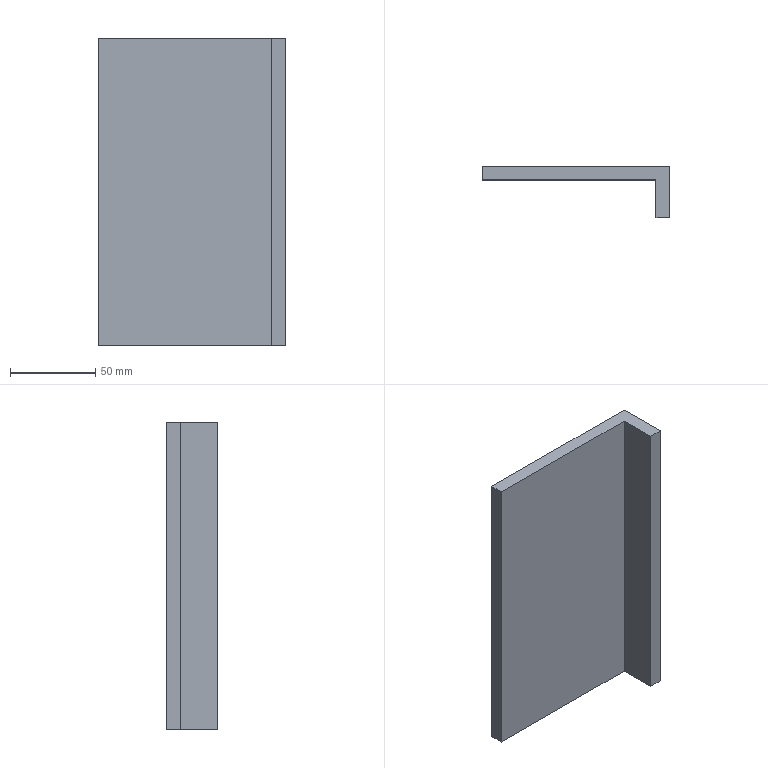Part | SolidWorks | features Extrusion 1 | 1 solid | 8 faces | box 110 x 30 x 180 mm | volume 190080 mm3 | plane 8
STEP:
#1=CARTESIAN_POINT('',(0.,0.,0.));
#2=VERTEX_POINT('',#1);
#3=CARTESIAN_POINT('',(0.,-8.,0.));
#4=VERTEX_POINT('',#3);
#5=CARTESIAN_POINT('',(0.,-8.,0.));
#6=DIRECTION('',(0.,-1.,0.));
#7=VECTOR('',#6,1000.);
#8=LINE('',#5,#7);
#9=EDGE_CURVE('',#2,#4,#8,.T.);
#10=ORIENTED_EDGE('',*,*,#9,.T.);
#11=CARTESIAN_POINT('',(0.,-8.,180.));
#12=VERTEX_POINT('',#11);
#13=CARTESIAN_POINT('',(0.,-8.,180.));
#14=DIRECTION('',(0.,0.,-1.));
#15=VECTOR('',#14,1000.);
#16=LINE('',#13,#15);
#17=EDGE_CURVE('',#12,#4,#16,.T.);
#18=ORIENTED_EDGE('',*,*,#17,.F.);
#19=CARTESIAN_POINT('',(0.,0.,180.));
#20=VERTEX_POINT('',#19);
#21=CARTESIAN_POINT('',(0.,-8.,180.));
#22=DIRECTION('',(0.,-1.,0.));
#23=VECTOR('',#22,1000.);
#24=LINE('',#21,#23);
#25=EDGE_CURVE('',#20,#12,#24,.T.);
#26=ORIENTED_EDGE('',*,*,#25,.F.);
#27=CARTESIAN_POINT('',(0.,0.,180.));
#28=DIRECTION('',(0.,0.,-1.));
#29=VECTOR('',#28,1000.);
#30=LINE('',#27,#29);
#31=EDGE_CURVE('',#20,#2,#30,.T.);
#32=ORIENTED_EDGE('',*,*,#31,.T.);
#33=EDGE_LOOP('',(#10,#18,#26,#32));
#34=FACE_OUTER_BOUND('',#33,.T.);
#35=CARTESIAN_POINT('',(0.,-8.,180.));
#36=DIRECTION('',(1.,0.,0.));
#37=DIRECTION('',(0.,0.,-1.));
#38=AXIS2_PLACEMENT_3D('',#35,#36,#37);
#39=PLANE('',#38);
#40=ADVANCED_FACE('',(#34),#39,.F.);
#41=CARTESIAN_POINT('',(102.,-8.,0.));
#42=VERTEX_POINT('',#41);
#43=CARTESIAN_POINT('',(0.,-8.,0.));
#44=DIRECTION('',(1.,0.,0.));
#45=VECTOR('',#44,1000.);
#46=LINE('',#43,#45);
#47=EDGE_CURVE('',#4,#42,#46,.T.);
#48=ORIENTED_EDGE('',*,*,#47,.T.);
#49=CARTESIAN_POINT('',(102.,-8.,180.));
#50=VERTEX_POINT('',#49);
#51=CARTESIAN_POINT('',(102.,-8.,180.));
#52=DIRECTION('',(0.,0.,-1.));
#53=VECTOR('',#52,1000.);
#54=LINE('',#51,#53);
#55=EDGE_CURVE('',#50,#42,#54,.T.);
#56=ORIENTED_EDGE('',*,*,#55,.F.);
#57=CARTESIAN_POINT('',(0.,-8.,180.));
#58=DIRECTION('',(1.,0.,0.));
#59=VECTOR('',#58,1000.);
#60=LINE('',#57,#59);
#61=EDGE_CURVE('',#12,#50,#60,.T.);
#62=ORIENTED_EDGE('',*,*,#61,.F.);
#63=ORIENTED_EDGE('',*,*,#17,.T.);
#64=EDGE_LOOP('',(#48,#56,#62,#63));
#65=FACE_OUTER_BOUND('',#64,.T.);
#66=CARTESIAN_POINT('',(0.,-8.,180.));
#67=DIRECTION('',(0.,1.,0.));
#68=DIRECTION('',(0.,0.,1.));
#69=AXIS2_PLACEMENT_3D('',#66,#67,#68);
#70=PLANE('',#69);
#71=ADVANCED_FACE('',(#65),#70,.F.);
#72=CARTESIAN_POINT('',(102.,-30.,0.));
#73=VERTEX_POINT('',#72);
#74=CARTESIAN_POINT('',(102.,-8.,0.));
#75=DIRECTION('',(0.,-1.,0.));
#76=VECTOR('',#75,1000.);
#77=LINE('',#74,#76);
#78=EDGE_CURVE('',#42,#73,#77,.T.);
#79=ORIENTED_EDGE('',*,*,#78,.T.);
#80=CARTESIAN_POINT('',(102.,-30.,180.));
#81=VERTEX_POINT('',#80);
#82=CARTESIAN_POINT('',(102.,-30.,180.));
#83=DIRECTION('',(0.,0.,-1.));
#84=VECTOR('',#83,1000.);
#85=LINE('',#82,#84);
#86=EDGE_CURVE('',#81,#73,#85,.T.);
#87=ORIENTED_EDGE('',*,*,#86,.F.);
#88=CARTESIAN_POINT('',(102.,-8.,180.));
#89=DIRECTION('',(0.,-1.,0.));
#90=VECTOR('',#89,1000.);
#91=LINE('',#88,#90);
#92=EDGE_CURVE('',#50,#81,#91,.T.);
#93=ORIENTED_EDGE('',*,*,#92,.F.);
#94=ORIENTED_EDGE('',*,*,#55,.T.);
#95=EDGE_LOOP('',(#79,#87,#93,#94));
#96=FACE_OUTER_BOUND('',#95,.T.);
#97=CARTESIAN_POINT('',(102.,-8.,180.));
#98=DIRECTION('',(1.,0.,0.));
#99=DIRECTION('',(0.,0.,-1.));
#100=AXIS2_PLACEMENT_3D('',#97,#98,#99);
#101=PLANE('',#100);
#102=ADVANCED_FACE('',(#96),#101,.F.);
#103=CARTESIAN_POINT('',(110.,-30.,0.));
#104=VERTEX_POINT('',#103);
#105=CARTESIAN_POINT('',(102.,-30.,0.));
#106=DIRECTION('',(1.,0.,0.));
#107=VECTOR('',#106,1000.);
#108=LINE('',#105,#107);
#109=EDGE_CURVE('',#73,#104,#108,.T.);
#110=ORIENTED_EDGE('',*,*,#109,.T.);
#111=CARTESIAN_POINT('',(110.,-30.,180.));
#112=VERTEX_POINT('',#111);
#113=CARTESIAN_POINT('',(110.,-30.,180.));
#114=DIRECTION('',(0.,0.,-1.));
#115=VECTOR('',#114,1000.);
#116=LINE('',#113,#115);
#117=EDGE_CURVE('',#112,#104,#116,.T.);
#118=ORIENTED_EDGE('',*,*,#117,.F.);
#119=CARTESIAN_POINT('',(102.,-30.,180.));
#120=DIRECTION('',(1.,0.,0.));
#121=VECTOR('',#120,1000.);
#122=LINE('',#119,#121);
#123=EDGE_CURVE('',#81,#112,#122,.T.);
#124=ORIENTED_EDGE('',*,*,#123,.F.);
#125=ORIENTED_EDGE('',*,*,#86,.T.);
#126=EDGE_LOOP('',(#110,#118,#124,#125));
#127=FACE_OUTER_BOUND('',#126,.T.);
#128=CARTESIAN_POINT('',(102.,-30.,180.));
#129=DIRECTION('',(0.,1.,0.));
#130=DIRECTION('',(0.,0.,1.));
#131=AXIS2_PLACEMENT_3D('',#128,#129,#130);
#132=PLANE('',#131);
#133=ADVANCED_FACE('',(#127),#132,.F.);
#134=CARTESIAN_POINT('',(110.,0.,0.));
#135=VERTEX_POINT('',#134);
#136=CARTESIAN_POINT('',(110.,0.,0.));
#137=DIRECTION('',(0.,1.,0.));
#138=VECTOR('',#137,1000.);
#139=LINE('',#136,#138);
#140=EDGE_CURVE('',#104,#135,#139,.T.);
#141=ORIENTED_EDGE('',*,*,#140,.T.);
#142=CARTESIAN_POINT('',(110.,0.,180.));
#143=VERTEX_POINT('',#142);
#144=CARTESIAN_POINT('',(110.,0.,180.));
#145=DIRECTION('',(0.,0.,-1.));
#146=VECTOR('',#145,1000.);
#147=LINE('',#144,#146);
#148=EDGE_CURVE('',#143,#135,#147,.T.);
#149=ORIENTED_EDGE('',*,*,#148,.F.);
#150=CARTESIAN_POINT('',(110.,0.,180.));
#151=DIRECTION('',(0.,1.,0.));
#152=VECTOR('',#151,1000.);
#153=LINE('',#150,#152);
#154=EDGE_CURVE('',#112,#143,#153,.T.);
#155=ORIENTED_EDGE('',*,*,#154,.F.);
#156=ORIENTED_EDGE('',*,*,#117,.T.);
#157=EDGE_LOOP('',(#141,#149,#155,#156));
#158=FACE_OUTER_BOUND('',#157,.T.);
#159=CARTESIAN_POINT('',(110.,0.,180.));
#160=DIRECTION('',(-1.,0.,0.));
#161=DIRECTION('',(0.,0.,1.));
#162=AXIS2_PLACEMENT_3D('',#159,#160,#161);
#163=PLANE('',#162);
#164=ADVANCED_FACE('',(#158),#163,.F.);
#165=CARTESIAN_POINT('',(0.,0.,0.));
#166=DIRECTION('',(-1.,0.,0.));
#167=VECTOR('',#166,1000.);
#168=LINE('',#165,#167);
#169=EDGE_CURVE('',#135,#2,#168,.T.);
#170=ORIENTED_EDGE('',*,*,#169,.T.);
#171=ORIENTED_EDGE('',*,*,#31,.F.);
#172=CARTESIAN_POINT('',(0.,0.,180.));
#173=DIRECTION('',(-1.,0.,0.));
#174=VECTOR('',#173,1000.);
#175=LINE('',#172,#174);
#176=EDGE_CURVE('',#143,#20,#175,.T.);
#177=ORIENTED_EDGE('',*,*,#176,.F.);
#178=ORIENTED_EDGE('',*,*,#148,.T.);
#179=EDGE_LOOP('',(#170,#171,#177,#178));
#180=FACE_OUTER_BOUND('',#179,.T.);
#181=CARTESIAN_POINT('',(0.,0.,180.));
#182=DIRECTION('',(0.,-1.,0.));
#183=DIRECTION('',(0.,0.,-1.));
#184=AXIS2_PLACEMENT_3D('',#181,#182,#183);
#185=PLANE('',#184);
#186=ADVANCED_FACE('',(#180),#185,.F.);
#187=ORIENTED_EDGE('',*,*,#25,.T.);
#188=ORIENTED_EDGE('',*,*,#61,.T.);
#189=ORIENTED_EDGE('',*,*,#92,.T.);
#190=ORIENTED_EDGE('',*,*,#123,.T.);
#191=ORIENTED_EDGE('',*,*,#154,.T.);
#192=ORIENTED_EDGE('',*,*,#176,.T.);
#193=EDGE_LOOP('',(#187,#188,#189,#190,#191,#192));
#194=FACE_OUTER_BOUND('',#193,.T.);
#195=CARTESIAN_POINT('',(0.,0.,180.));
#196=DIRECTION('',(0.,0.,-1.));
#197=DIRECTION('',(-1.,0.,0.));
#198=AXIS2_PLACEMENT_3D('',#195,#196,#197);
#199=PLANE('',#198);
#200=ADVANCED_FACE('',(#194),#199,.F.);
#201=ORIENTED_EDGE('',*,*,#9,.F.);
#202=ORIENTED_EDGE('',*,*,#169,.F.);
#203=ORIENTED_EDGE('',*,*,#140,.F.);
#204=ORIENTED_EDGE('',*,*,#109,.F.);
#205=ORIENTED_EDGE('',*,*,#78,.F.);
#206=ORIENTED_EDGE('',*,*,#47,.F.);
#207=EDGE_LOOP('',(#201,#202,#203,#204,#205,#206));
#208=FACE_OUTER_BOUND('',#207,.T.);
#209=CARTESIAN_POINT('',(0.,0.,0.));
#210=DIRECTION('',(0.,0.,-1.));
#211=DIRECTION('',(-1.,0.,0.));
#212=AXIS2_PLACEMENT_3D('',#209,#210,#211);
#213=PLANE('',#212);
#214=ADVANCED_FACE('',(#208),#213,.T.);
#215=CLOSED_SHELL('',(#40,#71,#102,#133,#164,#186,#200,#214));
#216=MANIFOLD_SOLID_BREP('',#215);
#217=CARTESIAN_POINT('',(0.,0.,0.));
#218=DIRECTION('',(0.,0.,1.));
#219=DIRECTION('',(1.,0.,0.));
#220=AXIS2_PLACEMENT_3D('',#217,#218,#219);
#221=(LENGTH_UNIT()NAMED_UNIT(*)SI_UNIT(.MILLI.,.METRE.));
#222=UNCERTAINTY_MEASURE_WITH_UNIT(LENGTH_MEASURE(0.00001),#221,'','');
#223=(NAMED_UNIT(*)PLANE_ANGLE_UNIT()SI_UNIT($,.RADIAN.));
#224=(NAMED_UNIT(*)SI_UNIT($,.STERADIAN.)SOLID_ANGLE_UNIT());
#225=(GEOMETRIC_REPRESENTATION_CONTEXT(3)GLOBAL_UNCERTAINTY_ASSIGNED_CONTEXT((#222))GLOBAL_UNIT_ASSIGNED_CONTEXT((#221,#223,#224))REPRESENTATION_CONTEXT('',''));
#226=ADVANCED_BREP_SHAPE_REPRESENTATION('',(#216,#220),#225);